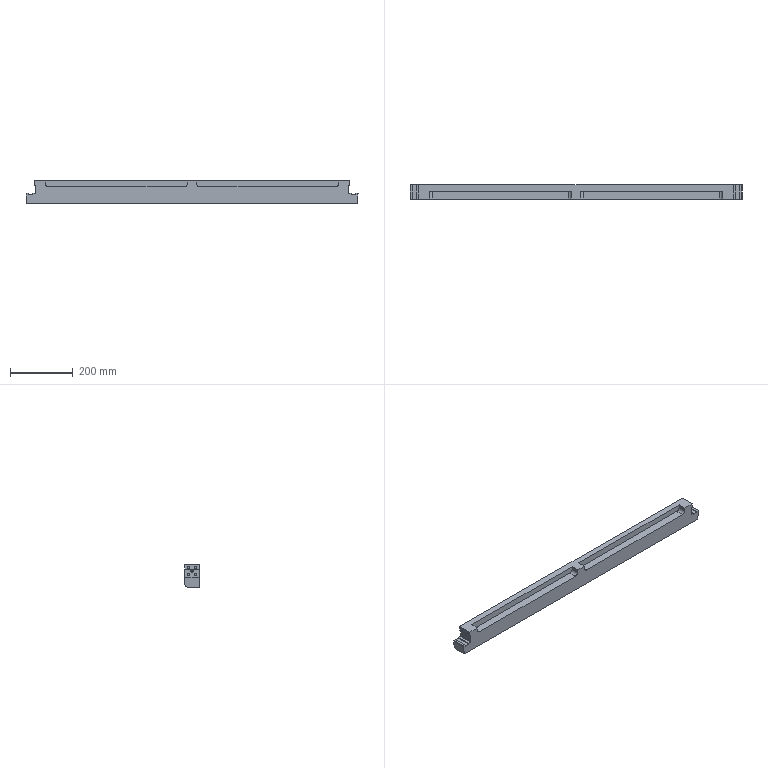NC program | NX | posted with a generic post | part box 1056 x 45 x 72.5 mm
Whole program:
N10 G17 G21 G94 G90
(ZLEVEL_PROFILE_COPY_1 , TOOL : D12)
N12 T20 M6
N14 G54
N16 G17 G0 G90 X532.563 Y44.63 B0. C0. S7500 M3
N18 G43 Z30. H20
N20 Z-1.
N22 G94 G1 X531.004 Y43.508 F3000.
N24 G3 X530.511 Y42.414 R1.2
N26 G1 X531.257 Y34.984
N28 X534.07 Y6.857
N30 X534.1 Y6.25
N32 Y4.25
N34 X534.096 Y3.509
N36 X534.097 Y-1.566
N38 G3 X534.697 Y-2.605 R1.2
N40 G1 X536.399 Y-3.588
N42 G0 Z-2.
N44 G1 X534.697 Y-2.605
N46 G2 X534.097 Y-1.566 R1.2
N48 G1 X534.096 Y3.509
N50 X534.1 Y4.25
N52 Y6.25
N54 X534.07 Y6.857
N56 X531.257 Y34.984
N58 X530.511 Y42.414
N60 G2 X531.004 Y43.508 R1.2
N62 G1 X532.563 Y44.63
N64 G0 Z-3.
N66 G1 X531.004 Y43.508
N68 G3 X530.511 Y42.414 R1.2
N70 G1 X531.257 Y34.984
N72 X534.07 Y6.857
N74 X534.1 Y6.25
N76 Y4.25
N78 X534.096 Y3.509
N80 X534.097 Y-1.566
N82 G3 X534.697 Y-2.605 R1.2
N84 G1 X536.399 Y-3.588
N86 G0 Z-4.
N88 G1 X534.697 Y-2.605
N90 G2 X534.097 Y-1.566 R1.2
N92 G1 X534.096 Y3.509
N94 X534.1 Y4.25
N96 Y6.25
N98 X534.07 Y6.857
N100 X531.257 Y34.984
N102 X530.511 Y42.414
N104 G2 X531.004 Y43.508 R1.2
N106 G1 X532.563 Y44.63
N108 G0 Z-5.
N110 G1 X531.004 Y43.508
N112 G3 X530.511 Y42.414 R1.2
N114 G1 X531.257 Y34.984
N116 X534.07 Y6.857
N118 X534.1 Y6.25
N120 Y4.25
N122 X534.096 Y3.509
N124 X534.097 Y-1.566
N126 G3 X534.697 Y-2.605 R1.2
N128 G1 X536.399 Y-3.588
N130 G0 Z-6.
N132 G1 X534.697 Y-2.605
N134 G2 X534.097 Y-1.566 R1.2
N136 G1 X534.096 Y3.509
N138 X534.1 Y4.25
N140 Y6.25
N142 X534.07 Y6.857
N144 X531.257 Y34.984
N146 X530.511 Y42.414
N148 G2 X531.004 Y43.508 R1.2
N150 G1 X532.563 Y44.63
N152 G0 Z-7.
N154 G1 X531.004 Y43.508
N156 G3 X530.511 Y42.414 R1.2
N158 G1 X531.257 Y34.984
N160 X534.07 Y6.857
N162 X534.1 Y6.25
N164 Y4.25
N166 X534.097 Y3.509
N168 Y-1.566
N170 G3 X534.697 Y-2.605 R1.2
N172 G1 X536.399 Y-3.588
N174 G0 Z-8.
N176 G1 X534.697 Y-2.605
N178 G2 X534.097 Y-1.566 R1.2
N180 G1 Y3.509
N182 X534.1 Y4.25
N184 Y6.25
N186 X534.07 Y6.857
N188 X531.257 Y34.984
N190 X530.511 Y42.414
N192 G2 X531.004 Y43.508 R1.2
N194 G1 X532.564 Y44.63
N196 G0 X532.571 Y44.635 Z-9.
N198 G1 X531.004 Y43.508
N200 G3 X530.511 Y42.414 R1.2
N202 G1 X531.257 Y34.984
N204 X534.07 Y6.857
N206 X534.1 Y6.25
N208 Y4.25
N210 X534.097 Y3.509
N212 Y-1.566
N214 G3 X534.697 Y-2.605 R1.2
N216 G1 X536.399 Y-3.588
N218 G0 X536.4 Z-10.
N220 G1 X534.697 Y-2.605
N222 G2 X534.097 Y-1.566 R1.2
N224 G1 Y3.509
N226 X534.1 Y4.25
N228 Y6.25
N230 X534.07 Y6.857
N232 X531.257 Y34.984
N234 X530.511 Y42.414
N236 G2 X531.005 Y43.508 R1.2
N238 G1 X532.571 Y44.635
N240 G0 Z-11.
N242 G1 X531.005 Y43.508
N244 G3 X530.511 Y42.414 R1.2
N246 G1 X531.257 Y34.984
N248 X534.07 Y6.857
N250 X534.1 Y6.25
N252 Y4.25
N254 X534.097 Y3.509
N256 Y-1.566
N258 G3 X534.697 Y-2.605 R1.2
N260 G1 X536.4 Y-3.588
N262 G0 Z-12.
N264 G1 X534.697 Y-2.605
N266 G2 X534.097 Y-1.566 R1.2
N268 G1 Y3.509
N270 X534.1 Y4.25
N272 Y6.25
N274 X534.07 Y6.857
N276 X531.257 Y34.984
N278 X530.511 Y42.414
N280 G2 X531.005 Y43.508 R1.2
N282 G1 X532.571 Y44.635
N284 G0 Z-13.
N286 G1 X531.005 Y43.508
N288 G3 X530.512 Y42.414 R1.2
N290 G1 X531.257 Y34.984
N292 X534.07 Y6.857
N294 X534.1 Y6.25
N296 Y4.25
N298 X534.097 Y3.509
N300 Y-1.566
N302 G3 X534.697 Y-2.605 R1.2
N304 G1 X536.4 Y-3.587
N306 G0 Z-14.
N308 G1 X534.698 Y-2.605
N310 G2 X534.097 Y-1.566 R1.2
N312 G1 Y3.509
N314 X534.1 Y4.25
N316 Y6.25
N318 X534.07 Y6.857
N320 X531.257 Y34.984
N322 X530.512 Y42.414
N324 G2 X531.005 Y43.508 R1.2
N326 G1 X532.571 Y44.635
N328 G0 Z-15.
N330 G1 X531.005 Y43.508
N332 G3 X530.512 Y42.414 R1.2
N334 G1 X531.257 Y34.984
N336 X534.07 Y6.857
N338 X534.1 Y6.25
N340 Y4.25
N342 X534.097 Y3.509
N344 Y-1.566
N346 G3 X534.698 Y-2.605 R1.2
N348 G1 X536.4 Y-3.587
N350 G0 Z-16.
N352 G1 X534.698 Y-2.605
N354 G2 X534.097 Y-1.566 R1.2
N356 G1 Y3.509
N358 X534.1 Y4.25
N360 Y6.25
N362 X534.07 Y6.857
N364 X531.257 Y34.984
N366 X530.512 Y42.414
N368 G2 X531.005 Y43.508 R1.2
N370 G1 X532.571 Y44.635
N372 G0 Y44.634 Z-17.
N374 G1 X531.005 Y43.508
N376 G3 X530.512 Y42.414 R1.2
N378 G1 X531.189 Y35.648
N380 X531.257 Y34.984
N382 X534.07 Y6.857
N384 X534.1 Y6.25
N386 Y4.25
N388 X534.097 Y3.509
N390 X534.098 Y-1.566
N392 G3 X534.698 Y-2.605 R1.2
N394 G1 X536.4 Y-3.587
N396 G0 Z-18.
N398 G1 X534.698 Y-2.605
N400 G2 X534.098 Y-1.566 R1.2
N402 G1 X534.097 Y3.509
N404 X534.1 Y4.25
N406 Y6.25
N408 X534.07 Y6.857
N410 X531.257 Y34.984
N412 X531.189 Y35.648
N414 X530.512 Y42.414
N416 G2 X531.006 Y43.508 R1.2
N418 G1 X532.571 Y44.634
N420 G0 Z-19.
N422 G1 X531.006 Y43.508
N424 G3 X530.512 Y42.414 R1.2
N426 G1 X531.189 Y35.648
N428 X531.257 Y34.984
N430 X534.07 Y6.857
N432 X534.1 Y6.25
N434 Y4.25
N436 X534.097 Y3.509
N438 X534.098 Y-1.566
N440 G3 X534.698 Y-2.605 R1.2
N442 G1 X536.4 Y-3.587
N444 G0 Z-20.
N446 G1 X534.698 Y-2.605
N448 G2 X534.098 Y-1.566 R1.2
N450 G1 X534.097 Y3.509
N452 X534.1 Y4.25
N454 Y6.25
N456 X534.07 Y6.857
N458 X531.257 Y34.984
N460 X531.189 Y35.648
N462 X530.512 Y42.414
N464 G2 X531.006 Y43.508 R1.2
N466 G1 X532.571 Y44.634
N468 G0 Z-21.
N470 G1 X531.006 Y43.508
N472 G3 X530.512 Y42.414 R1.2
N474 G1 X531.189 Y35.648
N476 X531.257 Y34.984
N478 X534.07 Y6.857
N480 X534.1 Y6.25
N482 Y4.25
N484 X534.097 Y3.509
N486 X534.098 Y-1.566
N488 G3 X534.698 Y-2.605 R1.2
N490 G1 X536.4 Y-3.587
N492 G0 Z-22.
N494 G1 X534.698 Y-2.605
N496 G2 X534.098 Y-1.566 R1.2
N498 G1 X534.097 Y3.509
N500 X534.1 Y4.25
N502 Y6.25
N504 X534.07 Y6.857
N506 X531.257 Y34.984
N508 X531.189 Y35.648
N510 X530.512 Y42.414
N512 G2 X531.006 Y43.508 R1.2
N514 G1 X532.571 Y44.634
N516 G0 X532.572 Z-23.
N518 G1 X531.006 Y43.508
N520 G3 X530.512 Y42.414 R1.2
N522 G1 X531.189 Y35.648
N524 X531.257 Y34.984
N526 X534.07 Y6.857
N528 X534.1 Y6.25
N530 Y4.25
N532 X534.097 Y3.509
N534 X534.098 Y-1.566
N536 G3 X534.698 Y-2.605 R1.2
N538 G1 X536.401 Y-3.587
N540 G0 Z-24.
N542 G1 X534.698 Y-2.605
N544 G2 X534.098 Y-1.566 R1.2
N546 G1 X534.097 Y3.509
N548 X534.1 Y4.25
N550 Y6.25
N552 X534.07 Y6.857
N554 X531.257 Y34.984
N556 X531.189 Y35.648
N558 X530.513 Y42.414
N560 G2 X531.006 Y43.508 R1.2
N562 G1 X532.572 Y44.634
N564 G0 Z-25.
N566 G1 X531.006 Y43.508
N568 G3 X530.513 Y42.414 R1.2
N570 G1 X531.189 Y35.648
N572 X531.257 Y34.984
N574 X534.07 Y6.857
N576 X534.1 Y6.25
N578 Y4.25
N580 X534.097 Y3.509
N582 X534.098 Y-1.566
N584 G3 X534.698 Y-2.605 R1.2
N586 G1 X536.401 Y-3.587
N588 G0 Z-26.
N590 G1 X534.698 Y-2.605
N592 G2 X534.098 Y-1.566 R1.2
N594 G1 X534.097 Y3.509
N596 X534.1 Y4.25
N598 Y6.25
N600 X534.07 Y6.857
N602 X531.251 Y35.029
N604 X530.513 Y42.414
N606 G2 X531.006 Y43.508 R1.2
N608 G1 X532.572 Y44.633
N610 G0 Y44.634 Z-27.
N612 G1 X531.006 Y43.508
N614 G3 X530.513 Y42.414 R1.2
N616 G1 X531.257 Y34.984
N618 X534.07 Y6.857
N620 X534.1 Y6.25
N622 Y4.25
N624 X534.097 Y3.509
N626 X534.098 Y-1.566
N628 G3 X534.698 Y-2.605 R1.2
N630 G1 X536.401 Y-3.587
N632 G0 Z-28.
N634 G1 X534.698 Y-2.605
N636 G2 X534.098 Y-1.566 R1.2
N638 G1 X534.097 Y3.509
N640 X534.1 Y4.25
N642 Y6.25
N644 X534.07 Y6.857
N646 X531.257 Y34.984
N648 X530.513 Y42.414
N650 G2 X531.006 Y43.508 R1.2
N652 G1 X532.572 Y44.634
N654 G0 Z-29.
N656 G1 X531.006 Y43.508
N658 G3 X530.513 Y42.414 R1.2
N660 G1 X531.257 Y34.984
N662 X534.07 Y6.857
N664 X534.1 Y6.25
N666 Y4.25
N668 X534.097 Y3.509
N670 X534.098 Y-1.566
N672 G3 X534.698 Y-2.605 R1.2
N674 G1 X536.401 Y-3.587
N676 G0 Z-30.
N678 G1 X534.699 Y-2.605
N680 G2 X534.098 Y-1.566 R1.2
N682 G1 X534.097 Y3.509
N684 X534.1 Y4.25
N686 Y6.25
N688 X534.07 Y6.857
N690 X531.257 Y34.984
N692 X530.513 Y42.414
N694 G2 X531.007 Y43.508 R1.2
N696 G1 X532.572 Y44.634
N698 G0 Z-31.
N700 G1 X531.007 Y43.508
N702 G3 X530.513 Y42.414 R1.2
N704 G1 X531.257 Y34.984
N706 X534.07 Y6.857
N708 X534.1 Y6.25
N710 Y4.25
N712 X534.097 Y3.509
N714 X534.098 Y-1.566
N716 G3 X534.699 Y-2.605 R1.2
N718 G1 X536.401 Y-3.587
N720 G0 Z-32.
N722 G1 X534.699 Y-2.605
N724 G2 X534.098 Y-1.566 R1.2
N726 G1 X534.097 Y3.509
N728 X534.1 Y4.25
N730 Y6.25
N732 X534.07 Y6.857
N734 X531.257 Y34.984
N736 X530.513 Y42.414
N738 G2 X531.007 Y43.508 R1.2
N740 G1 X532.572 Y44.634
N742 G0 Z-33.
N744 G1 X531.007 Y43.508
N746 G3 X530.513 Y42.415 R1.2
N748 G1 X531.257 Y34.984
N750 X534.07 Y6.857
N752 X534.1 Y6.25
N754 Y4.25
N756 X534.097 Y3.509
N758 X534.098 Y-1.566
N760 G3 X534.699 Y-2.605 R1.2
N762 G1 X536.401 Y-3.587
N764 G0 Z-34.
N766 G1 X534.699 Y-2.605
N768 G2 X534.098 Y-1.566 R1.2
N770 G1 X534.097 Y3.509
N772 X534.1 Y4.25
N774 Y6.25
N776 X534.07 Y6.857
N778 X531.257 Y34.984
N780 X530.513 Y42.415
N782 G2 X531.007 Y43.508 R1.2
N784 G1 X532.572 Y44.634
N786 G0 Y44.633 Z-35.
N788 G1 X531.007 Y43.508
N790 G3 X530.513 Y42.415 R1.2
N792 G1 X531.257 Y34.984
N794 X534.07 Y6.857
N796 X534.1 Y6.25
N798 Y4.25
N800 X534.097 Y3.509
N802 X534.098 Y-1.566
N804 G3 X534.699 Y-2.605 R1.2
N806 G1 X536.401 Y-3.587
N808 G0 Z-36.
N810 G1 X534.699 Y-2.605
N812 G2 X534.099 Y-1.566 R1.2
N814 G1 X534.097 Y3.509
N816 X534.1 Y4.25
N818 Y6.25
N820 X534.07 Y6.857
N822 X531.257 Y34.984
N824 X530.514 Y42.415
N826 G2 X531.007 Y43.508 R1.2
N828 G1 X532.572 Y44.633
N830 G0 Z-37.
N832 G1 X531.007 Y43.508
N834 G3 X530.514 Y42.415 R1.2
N836 G1 X531.257 Y34.984
N838 X534.07 Y6.857
N840 X534.1 Y6.25
N842 Y4.25
N844 X534.097 Y3.509
N846 X534.099 Y-1.566
N848 G3 X534.699 Y-2.605 R1.2
N850 G1 X536.402 Y-3.587
N852 G0 Z-38.
N854 G1 X534.699 Y-2.605
N856 G2 X534.099 Y-1.566 R1.2
N858 G1 X534.097 Y3.509
N860 X534.1 Y4.25
N862 Y6.25
N864 X534.07 Y6.857
N866 X531.257 Y34.984
N868 X530.514 Y42.415
N870 G2 X531.007 Y43.508 R1.2
N872 G1 X532.572 Y44.633
N874 G0 Z-39.
N876 G1 X531.007 Y43.508
N878 G3 X530.514 Y42.415 R1.2
N880 G1 X531.257 Y34.984
N882 X534.07 Y6.857
N884 X534.1 Y6.25
N886 Y4.25
N888 X534.097 Y3.509
N890 X534.099 Y-1.566
N892 G3 X534.699 Y-2.605 R1.2
N894 G1 X536.402 Y-3.587
N896 G0 Z-40.
N898 G1 X534.699 Y-2.605
N900 G2 X534.099 Y-1.566 R1.2
N902 G1 X534.097 Y3.509
N904 X534.1 Y4.25
N906 Y6.25
N908 X534.07 Y6.857
N910 X531.257 Y34.984
N912 X530.514 Y42.415
N914 G2 X531.008 Y43.508 R1.2
N916 G1 X532.572 Y44.633
N918 G0 Z-41.
N920 G1 X531.008 Y43.508
N922 G3 X530.514 Y42.415 R1.2
N924 G1 X531.257 Y34.984
N926 X534.07 Y6.857
N928 X534.1 Y6.25
N930 Y4.25
N932 X534.097 Y3.509
N934 X534.099 Y-1.566
N936 G3 X534.699 Y-2.605 R1.2
N938 G1 X536.402 Y-3.587
N940 G0 Z-42.
N942 G1 X534.699 Y-2.605
N944 G2 X534.099 Y-1.566 R1.2
N946 G1 X534.097 Y3.509
N948 X534.1 Y4.25
N950 Y6.25
N952 X534.07 Y6.857
N954 X531.257 Y34.984
N956 X530.514 Y42.415
N958 G2 X531.008 Y43.508 R1.2
N960 G1 X532.572 Y44.633
N962 G0 Z-43.
N964 G1 X531.008 Y43.508
N966 G3 X530.514 Y42.415 R1.2
N968 G1 X531.257 Y34.984
N970 X534.07 Y6.857
N972 X534.1 Y6.25
N974 Y4.25
N976 X534.097 Y3.509
N978 X534.099 Y-1.566
N980 G3 X534.699 Y-2.605 R1.2
N982 G1 X536.402 Y-3.587
N984 G0 Z-44.
N986 G1 X534.699 Y-2.605
N988 G2 X534.099 Y-1.566 R1.2
N990 G1 X534.097 Y3.509
N992 X534.1 Y4.25
N994 Y6.25
N996 X534.07 Y6.857
N998 X531.257 Y34.984
N1000 X530.514 Y42.415
N1002 G2 X531.008 Y43.508 R1.2
N1004 G1 X532.572 Y44.633
N1006 G0 Z-45.
N1008 G1 X531.008 Y43.508
N1010 G3 X530.514 Y42.415 R1.2
N1012 G1 X531.257 Y34.984
N1014 X534.07 Y6.857
N1016 X534.1 Y6.25
N1018 Y4.25
N1020 X534.097 Y3.509
N1022 X534.099 Y-1.566
N1024 G3 X534.699 Y-2.605 R1.2
N1026 G1 X536.402 Y-3.587
N1028 G0 Z30.
N1030 X-536.399 Y-3.588
N1032 Z-1.
N1034 G1 X-534.697 Y-2.605
N1036 G3 X-534.097 Y-1.566 R1.2
N1038 G1 X-534.096 Y3.35
N1040 X-534.1 Y4.204
N1042 Y6.25
N1044 G2 X-534.07 Y6.857 R6.1
N1046 G1 X-531.203 Y35.527
N1048 X-531.198 Y35.536
N1050 X-530.511 Y42.414
N1052 G3 X-531.004 Y43.508 R1.2
N1054 G1 X-532.576 Y44.638
N1056 G0 Z-2.
N1058 G1 X-531.004 Y43.508
N1060 G2 X-530.511 Y42.414 R1.2
N1062 G1 X-531.198 Y35.536
N1064 X-531.203 Y35.527
N1066 X-534.07 Y6.857
N1068 G3 X-534.1 Y6.25 R6.1
N1070 G1 Y4.204
N1072 X-534.096 Y3.35
N1074 X-534.097 Y-1.566
N1076 G2 X-534.697 Y-2.605 R1.2
N1078 G1 X-536.399 Y-3.588
N1080 G0 Z-3.
N1082 G1 X-534.697 Y-2.605
N1084 G3 X-534.097 Y-1.566 R1.2
N1086 G1 X-534.096 Y3.35
N1088 X-534.1 Y4.204
N1090 Y6.25
N1092 G2 X-534.07 Y6.857 R6.1
N1094 G1 X-531.203 Y35.527
N1096 X-531.198 Y35.536
N1098 X-530.511 Y42.414
N1100 G3 X-531.004 Y43.508 R1.2
N1102 G1 X-532.576 Y44.638
N1104 G0 Z-4.
N1106 G1 X-531.004 Y43.508
N1108 G2 X-530.511 Y42.414 R1.2
N1110 G1 X-531.198 Y35.536
N1112 X-531.203 Y35.527
N1114 X-534.07 Y6.857
N1116 G3 X-534.1 Y6.25 R6.1
N1118 G1 Y4.204
N1120 X-534.096 Y3.35
N1122 X-534.097 Y-1.566
N1124 G2 X-534.697 Y-2.605 R1.2
N1126 G1 X-536.399 Y-3.588
N1128 G0 Z-5.
N1130 G1 X-534.697 Y-2.605
N1132 G3 X-534.097 Y-1.566 R1.2
N1134 G1 X-534.096 Y3.35
N1136 X-534.1 Y4.204
N1138 Y6.25
N1140 G2 X-534.07 Y6.857 R6.1
N1142 G1 X-531.203 Y35.527
N1144 X-531.198 Y35.536
N1146 X-530.511 Y42.414
N1148 G3 X-531.005 Y43.508 R1.2
N1150 G1 X-532.576 Y44.638
N1152 G0 X-532.577 Z-6.
N1154 G1 X-531.005 Y43.508
N1156 G2 X-530.511 Y42.414 R1.2
N1158 G1 X-531.199 Y35.536
N1160 X-531.203 Y35.527
N1162 X-534.07 Y6.857
N1164 G3 X-534.1 Y6.25 R6.1
N1166 G1 Y4.204
N1168 X-534.096 Y3.35
N1170 X-534.097 Y-1.566
N1172 G2 X-534.697 Y-2.605 R1.2
N1174 G1 X-536.399 Y-3.588
N1176 G0 Z-7.
N1178 G1 X-534.697 Y-2.605
N1180 G3 X-534.097 Y-1.566 R1.2
N1182 G1 Y3.35
N1184 X-534.1 Y4.204
N1186 Y6.25
N1188 G2 X-534.07 Y6.857 R6.1
N1190 G1 X-531.203 Y35.527
N1192 X-531.199 Y35.536
N1194 X-530.511 Y42.414
N1196 G3 X-531.005 Y43.508 R1.2
N1198 G1 X-532.577 Y44.638
N1200 G0 Z-8.
N1202 G1 X-531.005 Y43.508
N1204 G2 X-530.511 Y42.414 R1.2
N1206 G1 X-531.199 Y35.536
N1208 X-531.203 Y35.527
N1210 X-534.07 Y6.857
N1212 G3 X-534.1 Y6.25 R6.1
N1214 G1 Y4.204
N1216 X-534.097 Y3.35
N1218 Y-1.566
N1220 G2 X-534.697 Y-2.605 R1.2
N1222 G1 X-536.399 Y-3.588
N1224 G0 Z-9.
N1226 G1 X-534.697 Y-2.605
N1228 G3 X-534.097 Y-1.566 R1.2
N1230 G1 Y3.35
N1232 X-534.1 Y4.204
N1234 Y6.25
N1236 G2 X-534.07 Y6.857 R6.1
N1238 G1 X-531.199 Y35.536
N1240 X-530.511 Y42.414
N1242 G3 X-531.005 Y43.508 R1.2
N1244 G1 X-532.577 Y44.638
N1246 G0 Z-10.
N1248 G1 X-531.005 Y43.508
N1250 G2 X-530.511 Y42.414 R1.2
N1252 G1 X-531.203 Y35.527
N1254 X-534.07 Y6.857
N1256 G3 X-534.1 Y6.25 R6.1
N1258 G1 Y4.204
N1260 X-534.097 Y3.35
N1262 Y-1.566
N1264 G2 X-534.697 Y-2.605 R1.2
N1266 G1 X-536.4 Y-3.588
N1268 G0 Z-11.
N1270 G1 X-534.697 Y-2.605
N1272 G3 X-534.097 Y-1.566 R1.2
N1274 G1 Y3.35
N1276 X-534.1 Y4.204
N1278 Y6.25
N1280 G2 X-534.07 Y6.857 R6.1
N1282 G1 X-531.199 Y35.536
N1284 X-530.511 Y42.414
N1286 G3 X-531.005 Y43.508 R1.2
N1288 G1 X-532.577 Y44.638
N1290 G0 Z-12.
N1292 G1 X-531.005 Y43.508
N1294 G2 X-530.511 Y42.414 R1.2
N1296 G1 X-531.203 Y35.527
N1298 X-534.07 Y6.857
N1300 G3 X-534.1 Y6.25 R6.1
N1302 G1 Y4.204
N1304 X-534.097 Y3.35
N1306 Y-1.566
N1308 G2 X-534.697 Y-2.605 R1.2
N1310 G1 X-536.4 Y-3.587
N1312 G0 Z-13.
N1314 G1 X-534.698 Y-2.605
N1316 G3 X-534.097 Y-1.566 R1.2
N1318 G1 Y3.35
N1320 X-534.1 Y4.204
N1322 Y6.25
N1324 G2 X-534.07 Y6.857 R6.1
N1326 G1 X-531.199 Y35.536
N1328 X-530.512 Y42.414
N1330 G3 X-531.005 Y43.508 R1.2
N1332 G1 X-532.577 Y44.638
N1334 G0 Z-14.
N1336 G1 X-531.005 Y43.508
N1338 G2 X-530.512 Y42.414 R1.2
N1340 G1 X-531.203 Y35.527
N1342 X-534.07 Y6.857
N1344 G3 X-534.1 Y6.25 R6.1
N1346 G1 Y4.204
N1348 X-534.097 Y3.35
N1350 Y-1.566
N1352 G2 X-534.698 Y-2.605 R1.2
N1354 G1 X-536.4 Y-3.587
N1356 G0 Z-15.
N1358 G1 X-534.698 Y-2.605
N1360 G3 X-534.097 Y-1.566 R1.2
N1362 G1 Y3.35
N1364 X-534.1 Y4.204
N1366 Y6.25
N1368 G2 X-534.07 Y6.857 R6.1
N1370 G1 X-531.199 Y35.536
N1372 X-530.512 Y42.414
N1374 G3 X-531.005 Y43.508 R1.2
N1376 G1 X-532.577 Y44.638
N1378 G0 X-532.578 Z-16.
N1380 G1 X-531.006 Y43.508
N1382 G2 X-530.512 Y42.414 R1.2
N1384 G1 X-531.203 Y35.527
N1386 X-534.07 Y6.857
N1388 G3 X-534.1 Y6.25 R6.1
N1390 G1 Y4.204
N1392 X-534.097 Y3.35
N1394 Y-1.566
N1396 G2 X-534.698 Y-2.605 R1.2
N1398 G1 X-536.4 Y-3.587
N1400 G0 Z-17.
N1402 G1 X-534.698 Y-2.605
N1404 G3 X-534.098 Y-1.566 R1.2
N1406 G1 X-534.097 Y3.35
N1408 X-534.1 Y4.204
N1410 Y6.25
N1412 G2 X-534.07 Y6.857 R6.1
N1414 G1 X-531.199 Y35.536
N1416 X-530.512 Y42.414
N1418 G3 X-531.006 Y43.508 R1.2
N1420 G1 X-532.578 Y44.638
N1422 G0 Z-18.
N1424 G1 X-531.006 Y43.508
N1426 G2 X-530.512 Y42.414 R1.2
N1428 G1 X-531.203 Y35.527
N1430 X-534.07 Y6.857
N1432 G3 X-534.1 Y6.25 R6.1
N1434 G1 Y4.204
N1436 X-534.097 Y3.35
N1438 X-534.098 Y-1.566
N1440 G2 X-534.698 Y-2.605 R1.2
N1442 G1 X-536.4 Y-3.587
N1444 G0 Z-19.
N1446 G1 X-534.698 Y-2.605
N1448 G3 X-534.098 Y-1.566 R1.2
N1450 G1 X-534.097 Y3.35
N1452 X-534.1 Y4.204
N1454 Y6.25
N1456 G2 X-534.07 Y6.857 R6.1
N1458 G1 X-531.2 Y35.536
N1460 X-530.512 Y42.414
N1462 G3 X-531.006 Y43.508 R1.2
N1464 G1 X-532.578 Y44.638
N1466 G0 Y44.639 Z-20.
N1468 G1 X-531.006 Y43.508
N1470 G2 X-530.512 Y42.414 R1.2
N1472 G1 X-531.203 Y35.514
N1474 X-531.323 Y34.326
N1476 X-534.07 Y6.857
N1478 G3 X-534.1 Y6.25 R6.1
N1480 G1 Y4.204
N1482 X-534.097 Y3.35
N1484 X-534.098 Y-1.566
N1486 G2 X-534.698 Y-2.605 R1.2
N1488 G1 X-536.4 Y-3.587
N1490 G0 Z-21.
N1492 G1 X-534.698 Y-2.605
N1494 G3 X-534.098 Y-1.566 R1.2
N1496 G1 X-534.097 Y3.35
N1498 X-534.1 Y4.204
N1500 Y6.25
N1502 G2 X-534.07 Y6.857 R6.1
N1504 G1 X-531.323 Y34.326
N1506 X-531.203 Y35.514
N1508 X-530.512 Y42.414
N1510 G3 X-531.006 Y43.508 R1.2
N1512 G1 X-532.578 Y44.639
N1514 G0 Z-22.
N1516 G1 X-531.006 Y43.508
N1518 G2 X-530.512 Y42.414 R1.2
N1520 G1 X-531.203 Y35.514
N1522 X-531.323 Y34.326
N1524 X-534.07 Y6.857
N1526 G3 X-534.1 Y6.25 R6.1
N1528 G1 Y4.204
N1530 X-534.097 Y3.35
N1532 X-534.098 Y-1.566
N1534 G2 X-534.698 Y-2.605 R1.2
N1536 G1 X-536.4 Y-3.587
N1538 G0 X-536.401 Z-23.
N1540 G1 X-534.698 Y-2.605
N1542 G3 X-534.098 Y-1.566 R1.2
N1544 G1 X-534.097 Y3.35
N1546 X-534.1 Y4.204
N1548 Y6.25
N1550 G2 X-534.07 Y6.857 R6.1
N1552 G1 X-531.323 Y34.326
N1554 X-531.203 Y35.514
N1556 X-530.512 Y42.414
N1558 G3 X-531.006 Y43.508 R1.2
N1560 G1 X-532.578 Y44.639
N1562 G0 Y44.638 Z-24.
N1564 G1 X-531.006 Y43.508
N1566 G2 X-530.513 Y42.414 R1.2
N1568 G1 X-531.274 Y34.802
N1570 X-531.323 Y34.326
N1572 X-534.07 Y6.857
N1574 G3 X-534.1 Y6.25 R6.1
N1576 G1 Y4.204
N1578 X-534.097 Y3.35
N1580 X-534.098 Y-1.566
N1582 G2 X-534.698 Y-2.605 R1.2
N1584 G1 X-536.401 Y-3.587
N1586 G0 Z-25.
N1588 G1 X-534.698 Y-2.605
N1590 G3 X-534.098 Y-1.566 R1.2
N1592 G1 X-534.097 Y3.35
N1594 X-534.1 Y4.204
N1596 Y6.25
N1598 G2 X-534.07 Y6.857 R6.1
N1600 G1 X-531.323 Y34.326
N1602 X-530.513 Y42.414
N1604 G3 X-531.006 Y43.508 R1.2
N1606 G1 X-532.578 Y44.639
N1608 G0 Z-26.
N1610 G1 X-531.006 Y43.508
N1612 G2 X-530.513 Y42.414 R1.2
N1614 G1 X-531.323 Y34.326
N1616 X-534.07 Y6.857
N1618 G3 X-534.1 Y6.25 R6.1
N1620 G1 Y4.204
N1622 X-534.097 Y3.35
N1624 X-534.098 Y-1.566
N1626 G2 X-534.698 Y-2.605 R1.2
N1628 G1 X-536.401 Y-3.587
N1630 G0 Z-27.
N1632 G1 X-534.698 Y-2.605
N1634 G3 X-534.098 Y-1.566 R1.2
N1636 G1 X-534.097 Y3.35
N1638 X-534.1 Y4.204
N1640 Y6.25
N1642 G2 X-534.07 Y6.857 R6.1
N1644 G1 X-531.323 Y34.326
N1646 X-530.513 Y42.414
N1648 G3 X-531.006 Y43.508 R1.2
N1650 G1 X-532.578 Y44.639
N1652 G0 X-532.579 Z-28.
N1654 G1 X-531.006 Y43.508
N1656 G2 X-530.513 Y42.414 R1.2
N1658 G1 X-531.323 Y34.326
N1660 X-534.07 Y6.857
N1662 G3 X-534.1 Y6.25 R6.1
N1664 G1 Y4.204
N1666 X-534.097 Y3.35
N1668 X-534.098 Y-1.566
N1670 G2 X-534.698 Y-2.605 R1.2
N1672 G1 X-536.401 Y-3.587
N1674 G0 Z-29.
N1676 G1 X-534.698 Y-2.605
N1678 G3 X-534.098 Y-1.566 R1.2
N1680 G1 X-534.097 Y3.35
N1682 X-534.1 Y4.204
N1684 Y6.25
N1686 G2 X-534.07 Y6.857 R6.1
N1688 G1 X-531.323 Y34.326
N1690 X-530.513 Y42.414
N1692 G3 X-531.006 Y43.508 R1.2
N1694 G1 X-532.579 Y44.639
N1696 G0 Z-30.
N1698 G1 X-531.007 Y43.508
N1700 G2 X-530.513 Y42.414 R1.2
N1702 G1 X-531.323 Y34.326
N1704 X-534.07 Y6.857
N1706 G3 X-534.1 Y6.25 R6.1
N1708 G1 Y4.204
N1710 X-534.097 Y3.35
N1712 X-534.098 Y-1.566
N1714 G2 X-534.699 Y-2.605 R1.2
N1716 G1 X-536.401 Y-3.587
N1718 G0 Z-31.
N1720 G1 X-534.699 Y-2.605
N1722 G3 X-534.098 Y-1.566 R1.2
N1724 G1 X-534.097 Y3.35
N1726 X-534.1 Y4.204
N1728 Y6.25
N1730 G2 X-534.07 Y6.857 R6.1
N1732 G1 X-531.323 Y34.326
N1734 X-530.513 Y42.414
N1736 G3 X-531.007 Y43.508 R1.2
N1738 G1 X-532.579 Y44.639
N1740 G0 Z-32.
N1742 G1 X-531.007 Y43.508
N1744 G2 X-530.513 Y42.414 R1.2
N1746 G1 X-531.323 Y34.326
N1748 X-534.07 Y6.857
N1750 G3 X-534.1 Y6.25 R6.1
N1752 G1 Y4.204
N1754 X-534.097 Y3.35
N1756 X-534.098 Y-1.566
N1758 G2 X-534.699 Y-2.605 R1.2
N1760 G1 X-536.401 Y-3.587
N1762 G0 Z-33.
N1764 G1 X-534.699 Y-2.605
N1766 G3 X-534.098 Y-1.566 R1.2
N1768 G1 X-534.097 Y3.35
N1770 X-534.1 Y4.204
N1772 Y6.25
N1774 G2 X-534.07 Y6.857 R6.1
N1776 G1 X-531.323 Y34.326
N1778 X-530.513 Y42.415
N1780 G3 X-531.007 Y43.508 R1.2
N1782 G1 X-532.579 Y44.639
N1784 G0 Z-34.
N1786 G1 X-531.007 Y43.508
N1788 G2 X-530.513 Y42.415 R1.2
N1790 G1 X-531.323 Y34.326
N1792 X-534.07 Y6.857
N1794 G3 X-534.1 Y6.25 R6.1
N1796 G1 Y4.204
N1798 X-534.097 Y3.35
N1800 X-534.098 Y-1.566
N1802 G2 X-534.699 Y-2.605 R1.2
N1804 G1 X-536.401 Y-3.587
N1806 G0 Z-35.
N1808 G1 X-534.699 Y-2.605
N1810 G3 X-534.098 Y-1.566 R1.2
N1812 G1 X-534.097 Y3.35
N1814 X-534.1 Y4.204
N1816 Y6.25
N1818 G2 X-534.07 Y6.857 R6.1
N1820 G1 X-531.323 Y34.326
N1822 X-530.513 Y42.415
N1824 G3 X-531.007 Y43.508 R1.2
N1826 G1 X-532.579 Y44.639
N1828 G0 Z-36.
N1830 G1 X-531.007 Y43.508
N1832 G2 X-530.514 Y42.415 R1.2
N1834 G1 X-531.323 Y34.326
N1836 X-534.07 Y6.857
N1838 G3 X-534.1 Y6.25 R6.1
N1840 G1 Y4.204
N1842 X-534.097 Y3.35
N1844 X-534.099 Y-1.566
N1846 G2 X-534.699 Y-2.605 R1.2
N1848 G1 X-536.402 Y-3.587
N1850 G0 Z-37.
N1852 G1 X-534.699 Y-2.605
N1854 G3 X-534.099 Y-1.566 R1.2
N1856 G1 X-534.097 Y3.35
N1858 X-534.1 Y4.204
N1860 Y6.25
N1862 G2 X-534.07 Y6.857 R6.1
N1864 G1 X-531.323 Y34.326
N1866 X-530.514 Y42.415
N1868 G3 X-531.007 Y43.508 R1.2
N1870 G1 X-532.58 Y44.639
N1872 G0 Z-38.
N1874 G1 X-531.007 Y43.508
N1876 G2 X-530.514 Y42.415 R1.2
N1878 G1 X-531.323 Y34.326
N1880 X-534.07 Y6.857
N1882 G3 X-534.1 Y6.25 R6.1
N1884 G1 Y4.204
N1886 X-534.097 Y3.35
N1888 X-534.099 Y-1.566
N1890 G2 X-534.699 Y-2.605 R1.2
N1892 G1 X-536.402 Y-3.587
N1894 G0 Z-39.
N1896 G1 X-534.699 Y-2.605
N1898 G3 X-534.099 Y-1.566 R1.2
N1900 G1 X-534.097 Y3.35
N1902 X-534.1 Y4.204
N1904 Y6.25
N1906 G2 X-534.07 Y6.857 R6.1
N1908 G1 X-531.323 Y34.326
N1910 X-530.514 Y42.415
N1912 G3 X-531.007 Y43.508 R1.2
N1914 G1 X-532.58 Y44.639
N1916 G0 Z-40.
N1918 G1 X-531.008 Y43.508
N1920 G2 X-530.514 Y42.415 R1.2
N1922 G1 X-531.202 Y35.533
N1924 X-534.07 Y6.857
N1926 G3 X-534.1 Y6.25 R6.1
N1928 G1 Y4.204
N1930 G3 X-534.042 Y3.411 R6.1
N1932 G1 X-534.097 Y3.35
N1934 X-534.099 Y-1.566
N1936 G2 X-534.699 Y-2.605 R1.2
N1938 G1 X-536.402 Y-3.587
N1940 G0 Z-41.
N1942 G1 X-534.699 Y-2.605
N1944 G3 X-534.099 Y-1.566 R1.2
N1946 G1 X-534.097 Y3.35
N1948 X-534.042 Y3.411
N1950 G2 X-534.1 Y4.25 R6.1
N1952 G1 Y6.25
N1954 G2 X-534.07 Y6.857 R6.1
N1956 G1 X-531.202 Y35.533
N1958 X-530.514 Y42.415
N1960 G3 X-531.008 Y43.508 R1.2
N1962 G1 X-532.58 Y44.639
N1964 G0 Z-42.
N1966 G1 X-531.008 Y43.508
N1968 G2 X-530.514 Y42.415 R1.2
N1970 G1 X-531.202 Y35.533
N1972 X-534.07 Y6.857
N1974 G3 X-534.1 Y6.25 R6.1
N1976 G1 Y4.204
N1978 G3 X-534.042 Y3.411 R6.1
N1980 G1 X-534.097 Y3.35
N1982 X-534.099 Y-1.566
N1984 G2 X-534.699 Y-2.605 R1.2
N1986 G1 X-536.402 Y-3.587
N1988 G0 Z-43.
N1990 G1 X-534.699 Y-2.605
N1992 G3 X-534.099 Y-1.566 R1.2
N1994 G1 X-534.097 Y3.35
N1996 X-534.042 Y3.411
N1998 G2 X-534.1 Y4.25 R6.1
N2000 G1 Y6.25
N2002 G2 X-534.07 Y6.857 R6.1
N2004 G1 X-531.202 Y35.533
N2006 X-530.514 Y42.415
N2008 G3 X-531.008 Y43.508 R1.2
N2010 G1 X-532.58 Y44.639
N2012 G0 Z-44.
N2014 G1 X-531.008 Y43.508
N2016 G2 X-530.514 Y42.415 R1.2
N2018 G1 X-531.202 Y35.533
N2020 X-534.07 Y6.857
N2022 G3 X-534.1 Y6.25 R6.1
N2024 G1 Y4.204
N2026 G3 X-534.042 Y3.411 R6.1
N2028 G1 X-534.097 Y3.35
N2030 X-534.099 Y-1.566
N2032 G2 X-534.699 Y-2.605 R1.2
N2034 G1 X-536.402 Y-3.587
N2036 G0 Z-45.
N2038 G1 X-534.699 Y-2.605
N2040 G3 X-534.099 Y-1.566 R1.2
N2042 G1 X-534.097 Y3.35
N2044 X-534.042 Y3.411
N2046 G2 X-534.1 Y4.25 R6.1
N2048 G1 Y6.25
N2050 G2 X-534.07 Y6.857 R6.1
N2052 G1 X-531.202 Y35.533
N2054 X-530.514 Y42.415
N2056 G3 X-531.008 Y43.508 R1.2
N2058 G1 X-532.58 Y44.639
N2060 G0 Z30.
N2062 M5
(111 , TOOL : D12JING)
N2064 T21 M6
N2066 G54
N2068 G17 G0 G90 X524.294 Y47.768 B0. C0. S6500 M3
N2070 G43 Z30. H21
N2072 Z-14.
N2074 G94 G1 Z-15. F1000.
N2076 G41 X524.227 Y47.693 D21
N2078 X523.519 Y46.566
N2080 G3 X523.73 Y45.038 R1.2
N2082 G1 X528.844 Y40.411
N2084 X529.076 Y40.201
N2086 G2 X531.02 Y36.35 R6.
N2088 G1 X533.97 Y6.847
N2090 X534. Y6.25
N2092 Y4.789
N2094 X534.002 Y4.765
N2096 X533.978 Y4.76
N2098 G2 X532.243 Y0.007 R6.
N2100 G1 X531.743 Y-0.493
N2102 X531.379 Y-0.854
N2104 X527.195 Y-5.038
N2106 G3 X527.06 Y-6.575 R1.2
N2108 G1 X527.828 Y-7.671
N2110 G40
N2112 X527.899 Y-7.742
N2114 Z-14.
N2116 G0 Z30.
N2118 X524.295 Y47.768
N2120 Z-29.
N2122 G1 Z-30.
N2124 G41 X524.227 Y47.694
N2126 X523.519 Y46.567
N2128 G3 X523.73 Y45.038 R1.2
N2130 G1 X528.844 Y40.411
N2132 X529.076 Y40.201
N2134 G2 X531.02 Y36.35 R6.
N2136 G1 X533.97 Y6.847
N2138 X534. Y6.25
N2140 Y4.789
N2142 X534.002 Y4.765
N2144 X533.978 Y4.76
N2146 G2 X532.243 Y0.007 R6.
N2148 G1 X531.743 Y-0.493
N2150 X531.379 Y-0.855
N2152 X527.196 Y-5.038
N2154 G3 X527.061 Y-6.575 R1.2
N2156 G1 X527.828 Y-7.671
N2158 G40
N2160 X527.899 Y-7.742
N2162 Z-29.
N2164 G0 Z30.
N2166 X524.295 Y47.768
N2168 Z-44.
N2170 G1 Z-45.
N2172 G41 X524.228 Y47.694
N2174 X523.52 Y46.567
N2176 G3 X523.73 Y45.039 R1.2
N2178 G1 X528.844 Y40.411
N2180 X529.076 Y40.201
N2182 G2 X531.02 Y36.35 R6.
N2184 G1 X533.97 Y6.847
N2186 X534. Y6.25
N2188 Y4.868
N2190 X533.999 Y4.762
N2192 X533.98 Y4.745
N2194 G2 X532.243 Y0.007 R6.
N2196 G1 X531.743 Y-0.493
N2198 X527.196 Y-5.039
N2200 G3 X527.061 Y-6.576 R1.2
N2202 G1 X527.829 Y-7.672
N2204 G40
N2206 X527.9 Y-7.743
N2208 Z-44.
N2210 G0 Z30.
N2212 X-527.898 Y-7.741
N2214 Z-14.
N2216 G1 Z-15.
N2218 G41 X-527.828 Y-7.671
N2220 X-527.06 Y-6.574
N2222 G3 X-527.195 Y-5.038 R1.2
N2224 G1 X-531.474 Y-0.758
N2226 X-531.743 Y-0.493
N2228 X-531.775 Y-0.46
N2230 X-531.781 Y-0.449
N2232 X-531.868 Y-0.366
N2234 X-531.857 Y-0.346
N2236 G2 X-534. Y4.25 R6.
N2238 G1 Y6.25
N2240 G2 X-533.97 Y6.847 R6.
N2242 G1 X-531.02 Y36.35
N2244 G2 X-529.076 Y40.201 R6.
N2246 G1 X-528.81 Y40.442
N2248 X-523.73 Y45.038
N2250 G3 X-523.518 Y46.566 R1.2
N2252 G1 X-524.227 Y47.693
N2254 G40
N2256 X-524.294 Y47.767
N2258 Z-14.
N2260 G0 Z30.
N2262 X-527.898 Y-7.742
N2264 Z-29.
N2266 G1 Z-30.
N2268 G41 X-527.827 Y-7.671
N2270 X-527.06 Y-6.575
N2272 G3 X-527.195 Y-5.038 R1.2
N2274 G1 X-531.743 Y-0.493
N2276 X-531.775 Y-0.46
N2278 X-531.781 Y-0.449
N2280 X-531.868 Y-0.367
N2282 X-531.857 Y-0.346
N2284 G2 X-534. Y4.25 R6.
N2286 G1 Y6.25
N2288 G2 X-533.97 Y6.847 R6.
N2290 G1 X-531.02 Y36.35
N2292 G2 X-529.076 Y40.201 R6.
N2294 G1 X-528.81 Y40.442
N2296 X-523.73 Y45.038
N2298 G3 X-523.519 Y46.566 R1.2
N2300 G1 X-524.227 Y47.694
N2302 G40
N2304 X-524.294 Y47.768
N2306 Z-29.
N2308 G0 Z30.
N2310 X-527.898 Y-7.742
N2312 Z-44.
N2314 G1 Z-45.
N2316 G41 X-527.828 Y-7.671
N2318 X-527.06 Y-6.575
N2320 G3 X-527.195 Y-5.038 R1.2
N2322 G1 X-531.743 Y-0.493
N2324 X-531.775 Y-0.46
N2326 X-531.782 Y-0.449
N2328 X-531.868 Y-0.367
N2330 X-531.857 Y-0.346
N2332 G2 X-534. Y4.25 R6.
N2334 G1 Y6.25
N2336 G2 X-533.97 Y6.847 R6.
N2338 G1 X-531.02 Y36.35
N2340 G2 X-529.076 Y40.201 R6.
N2342 G1 X-528.81 Y40.442
N2344 X-528.448 Y40.768
N2346 X-523.73 Y45.038
N2348 G3 X-523.519 Y46.566 R1.2
N2350 G1 X-524.228 Y47.694
N2352 G40
N2354 X-524.295 Y47.768
N2356 Z-44.
N2358 G0 Z30.
N2360 M5
(FLOOR_WALL_1 , TOOL : D10)
N2362 T10 M6
N2364 G54
N2366 G17 G0 G90 X-38.519 Y-44.25 B0. C0. S7500 M3
N2368 G43 Z30. H10
N2370 Z-21.85
N2372 G94 G1 Z-24.85 F1000.
N2374 X-39.053 Y-41.25
N2376 G2 X-39.157 Y-40.6 R19.2 F3000.
N2378 G1 X-441.843
N2380 G2 X-441.948 Y-41.25 R19.2
N2382 G1 X-442.761
N2384 G3 X-442.55 Y-39.8 R18.4
N2386 G1 X-38.45
N2388 G3 X-38.24 Y-41.25 R18.4
N2390 G1 X-37.426
N2392 G2 X-37.715 Y-39. R17.6
N2394 G1 X-443.285
N2396 G2 X-443.575 Y-41.25 R17.6
N2398 G1 X-444.391
N2400 G3 X-444.053 Y-38.2 R16.8
N2402 G1 X-36.947
N2404 G3 X-36.61 Y-41.25 R16.8
N2406 G1 X-35.792
N2408 G2 X-36.15 Y-37.877 R16.
N2410 G1 Y-37.4
N2412 X-444.85
N2414 Y-37.883
N2416 G2 X-445.208 Y-41.25 R16.
N2418 G1 X-446.028
N2420 G3 X-445.65 Y-37.883 R15.2
N2422 G1 Y-36.6
N2424 X-35.35
N2426 Y-37.877
N2428 G3 X-34.973 Y-41.25 R15.2
N2430 G1 X-34.152
N2432 G2 X-34.55 Y-37.877 R14.4
N2434 G1 Y-35.8
N2436 X-446.45
N2438 Y-37.883
N2440 G2 X-446.849 Y-41.25 R14.4
N2442 G1 X-447.673
N2444 G3 X-447.25 Y-37.883 R13.6
N2446 G1 Y-35.
N2448 X-33.75
N2450 Y-37.877
N2452 G3 X-33.328 Y-41.25 R13.6
N2454 G1 X-32.5
N2456 G2 X-32.95 Y-37.877 R12.8
N2458 G1 Y-34.2
N2460 X-448.05
N2462 Y-37.883
N2464 G2 X-448.501 Y-41.25 R12.8
N2466 G1 X-449.332
N2468 G3 X-448.85 Y-37.883 R12.
N2470 G1 Y-33.4
N2472 X-32.15
N2474 Y-37.877
N2476 G3 X-31.669 Y-41.25 R12.
N2478 G1 X-30.833
N2480 G2 X-31.35 Y-37.877 R11.2
N2482 G1 Y-32.6
N2484 X-449.65
N2486 Y-37.883
N2488 G2 X-450.168 Y-41.25 R11.2
N2490 G1 X-451.01
N2492 G3 X-450.45 Y-37.883 R10.4
N2494 G1 Y-31.8
N2496 X-30.55
N2498 Y-37.877
N2500 G3 X-29.991 Y-41.25 R10.4
N2502 G1 X-29.142
N2504 G2 X-29.75 Y-37.877 R9.6
N2506 G1 Y-31.
N2508 X-451.25
N2510 Y-37.883
N2512 G2 X-451.86 Y-41.25 R9.6
N2514 G1 X-452.72
N2516 G3 X-452.05 Y-37.883 R8.8
N2518 G1 Y-30.2
N2520 X-28.95
N2522 Y-37.877
N2524 G3 X-28.282 Y-41.25 R8.8
N2526 G1 X-27.409
N2528 G2 X-28.15 Y-37.878 R8.
N2530 G1 Y-29.4
N2532 X-452.85
N2534 Y-37.883
N2536 G2 X-453.593 Y-41.25 R8.
N2538 G1 X-454.486
N2540 G3 X-453.65 Y-37.883 R7.2
N2542 G1 Y-28.6
N2544 X-27.35
N2546 Y-37.878
N2548 G3 X-26.516 Y-41.25 R7.2
N2550 G1 X-25.595
N2552 G2 X-26.55 Y-37.878 R6.4
N2554 G1 Y-27.8
N2556 X-454.45
N2558 Y-37.883
N2560 G2 X-455.407 Y-41.25 R6.4
N2562 G1 X-456.375
N2564 G3 X-455.25 Y-37.883 R5.6
N2566 G1 Y-27.
N2568 X-25.75
N2570 Y-37.879
N2572 G3 X-24.627 Y-41.25 R5.6
N2574 G1 X-23.571
N2576 X-23.648 Y-41.174
N2578 G2 X-24.95 Y-37.879 R4.8
N2580 G1 Y-26.25
N2582 X-24.947 Y-26.197
N2584 X-25. Y-26.2
N2586 X-456.
N2588 X-456.053 Y-26.197
N2590 X-456.05 Y-26.25
N2592 Y-37.883
N2594 G2 X-457.429 Y-41.25 R4.8
N2596 G1 X-458.56
N2598 X-458.022 Y-40.712
N2600 G3 X-456.85 Y-37.883 R4.
N2602 G1 Y-26.25
N2604 G2 X-456. Y-25.4 R0.85
N2606 G1 X-25.
N2608 G2 X-24.15 Y-26.25 R0.85
N2610 G1 Y-37.88
N2612 G3 X-23.072 Y-40.618 R4.
N2614 G1 X-22.44 Y-41.25
N2616 X-21.309
N2618 X-22.496 Y-40.063
N2620 G2 X-23.35 Y-37.88 R3.2
N2622 G1 Y-26.25
N2624 G3 X-25. Y-24.6 R1.65
N2626 G1 X-456.
N2628 G3 X-457.65 Y-26.25 R1.65
N2630 G1 Y-37.883
N2632 G2 X-458.587 Y-40.146 R3.2
N2634 G1 X-459.691 Y-41.25
N2636 X-460.823
N2638 X-459.153 Y-39.58
N2640 G3 X-458.45 Y-37.883 R2.4
N2642 G1 Y-26.25
N2644 G2 X-456. Y-23.8 R2.45
N2646 G1 X-25.
N2648 G2 X-22.55 Y-26.25 R2.45
N2650 G1 Y-37.881
N2652 G3 X-21.918 Y-39.509 R2.4
N2654 G1 X-20.177 Y-41.25
N2656 X-19.046
N2658 X-21.338 Y-38.958
N2660 G2 X-21.75 Y-37.882 R1.6
N2662 G1 Y-26.25
N2664 G3 X-25. Y-23. R3.25
N2666 G1 X-456.
N2668 G3 X-459.25 Y-26.25 R3.25
N2670 G1 Y-37.883
N2672 G2 X-459.719 Y-39.015 R1.6
N2674 G1 X-461.954 Y-41.25
N2676 X-463.085
N2678 X-460.284 Y-38.449
N2680 G3 X-460.05 Y-37.883 R0.8
N2682 G1 Y-26.25
N2684 G2 X-456. Y-22.2 R4.05
N2686 G1 X-25.
N2688 G2 X-20.95 Y-26.25 R4.05
N2690 G1 Y-37.883
N2692 G3 X-20.753 Y-38.412 R0.8
N2694 G1 X-17.915 Y-41.25
N2696 X-16.813
N2698 Y-41.22
N2700 X-20.15 Y-37.883
N2702 Y-26.25
N2704 G3 X-25. Y-21.4 R4.85
N2706 G1 X-456.
N2708 G3 X-460.85 Y-26.25 R4.85
N2710 G1 Y-37.883
N2712 X-464.217 Y-41.25
N2714 X-467.367 Y-44.4
N2716 Z-21.85
N2718 G0 Z30.
N2720 X442.481 Y-44.25
N2722 Z-21.85
N2724 G1 Z-24.85 F1000.
N2726 X441.947 Y-41.25
N2728 G2 X441.843 Y-40.6 R19.2 F3000.
N2730 G1 X39.157
N2732 G2 X39.053 Y-41.25 R19.2
N2734 G1 X38.239
N2736 G3 X38.45 Y-39.8 R18.4
N2738 G1 X442.55
N2740 G3 X442.76 Y-41.25 R18.4
N2742 G1 X443.574
N2744 G2 X443.285 Y-39. R17.6
N2746 G1 X37.715
N2748 G2 X37.425 Y-41.25 R17.6
N2750 G1 X36.609
N2752 G3 X36.947 Y-38.2 R16.8
N2754 G1 X444.053
N2756 G3 X444.39 Y-41.25 R16.8
N2758 G1 X445.208
N2760 G2 X444.85 Y-37.876 R16.
N2762 G1 Y-37.4
N2764 X36.15
N2766 Y-37.883
N2768 G2 X35.792 Y-41.25 R16.
N2770 G1 X34.972
N2772 G3 X35.35 Y-37.883 R15.2
N2774 G1 Y-36.6
N2776 X445.65
N2778 Y-37.876
N2780 G3 X446.027 Y-41.25 R15.2
N2782 G1 X446.848
N2784 G2 X446.45 Y-37.876 R14.4
N2786 G1 Y-35.8
N2788 X34.55
N2790 Y-37.883
N2792 G2 X34.151 Y-41.25 R14.4
N2794 G1 X33.327
N2796 G3 X33.75 Y-37.883 R13.6
N2798 G1 Y-35.
N2800 X447.25
N2802 Y-37.876
N2804 G3 X447.672 Y-41.25 R13.6
N2806 G1 X448.5
N2808 G2 X448.05 Y-37.876 R12.8
N2810 G1 Y-34.2
N2812 X32.95
N2814 Y-37.883
N2816 G2 X32.499 Y-41.25 R12.8
N2818 G1 X31.668
N2820 G3 X32.15 Y-37.883 R12.
N2822 G1 Y-33.4
N2824 X448.85
N2826 Y-37.876
N2828 G3 X449.331 Y-41.25 R12.
N2830 G1 X450.167
N2832 G2 X449.65 Y-37.876 R11.2
N2834 G1 Y-32.6
N2836 X31.35
N2838 Y-37.883
N2840 G2 X30.832 Y-41.25 R11.2
N2842 G1 X29.99
N2844 G3 X30.55 Y-37.883 R10.4
N2846 G1 Y-31.8
N2848 X450.45
N2850 Y-37.876
N2852 G3 X451.009 Y-41.25 R10.4
N2854 G1 X451.859
N2856 G2 X451.25 Y-37.876 R9.6
N2858 G1 Y-31.
N2860 X29.75
N2862 Y-37.883
N2864 G2 X29.14 Y-41.25 R9.6
N2866 G1 X28.28
N2868 G3 X28.95 Y-37.883 R8.8
N2870 G1 Y-30.2
N2872 X452.05
N2874 Y-37.877
N2876 G3 X452.718 Y-41.25 R8.8
N2878 G1 X453.591
N2880 G2 X452.85 Y-37.877 R8.
N2882 G1 Y-29.4
N2884 X28.15
N2886 Y-37.883
N2888 G2 X27.407 Y-41.25 R8.
N2890 G1 X26.514
N2892 G3 X27.35 Y-37.883 R7.2
N2894 G1 Y-28.6
N2896 X453.65
N2898 Y-37.877
N2900 G3 X454.484 Y-41.25 R7.2
N2902 G1 X455.405
N2904 G2 X454.45 Y-37.878 R6.4
N2906 G1 Y-27.8
N2908 X26.55
N2910 Y-37.883
N2912 G2 X25.593 Y-41.25 R6.4
N2914 G1 X24.625
N2916 G3 X25.75 Y-37.883 R5.6
N2918 G1 Y-27.
N2920 X455.25
N2922 Y-37.878
N2924 G3 X456.373 Y-41.25 R5.6
N2926 G1 X457.429
N2928 X457.352 Y-41.174
N2930 G2 X456.05 Y-37.879 R4.8
N2932 G1 Y-26.25
N2934 X456.053 Y-26.197
N2936 X456. Y-26.2
N2938 X25.
N2940 X24.947 Y-26.197
N2942 X24.95 Y-26.25
N2944 Y-37.883
N2946 G2 X23.571 Y-41.25 R4.8
N2948 G1 X22.44
N2950 X22.978 Y-40.712
N2952 G3 X24.15 Y-37.883 R4.
N2954 G1 Y-26.25
N2956 G2 X25. Y-25.4 R0.85
N2958 G1 X456.
N2960 G2 X456.85 Y-26.25 R0.85
N2962 G1 Y-37.88
N2964 G3 X457.928 Y-40.618 R4.
N2966 G1 X458.56 Y-41.25
N2968 X459.691
N2970 X458.504 Y-40.063
N2972 G2 X457.65 Y-37.88 R3.2
N2974 G1 Y-26.25
N2976 G3 X456. Y-24.6 R1.65
N2978 G1 X25.
N2980 G3 X23.35 Y-26.25 R1.65
N2982 G1 Y-37.883
N2984 G2 X22.413 Y-40.146 R3.2
N2986 G1 X21.309 Y-41.25
N2988 X20.177
N2990 X21.847 Y-39.58
N2992 G3 X22.55 Y-37.883 R2.4
N2994 G1 Y-26.25
N2996 G2 X25. Y-23.8 R2.45
N2998 G1 X456.
N3000 G2 X458.45 Y-26.25 R2.45
N3002 G1 Y-37.881
N3004 G3 X459.082 Y-39.509 R2.4
N3006 G1 X460.823 Y-41.25
N3008 X461.954
N3010 X459.662 Y-38.958
N3012 G2 X459.25 Y-37.882 R1.6
N3014 G1 Y-26.25
N3016 G3 X456. Y-23. R3.25
N3018 G1 X25.
N3020 G3 X21.75 Y-26.25 R3.25
N3022 G1 Y-37.883
N3024 G2 X21.281 Y-39.015 R1.6
N3026 G1 X19.046 Y-41.25
N3028 X17.915
N3030 X20.716 Y-38.449
N3032 G3 X20.95 Y-37.883 R0.8
N3034 G1 Y-26.25
N3036 G2 X25. Y-22.2 R4.05
N3038 G1 X456.
N3040 G2 X460.05 Y-26.25 R4.05
N3042 G1 Y-37.883
N3044 G3 X460.247 Y-38.412 R0.8
N3046 G1 X463.085 Y-41.25
N3048 X464.187
N3050 Y-41.22
N3052 X460.85 Y-37.883
N3054 Y-26.25
N3056 G3 X456. Y-21.4 R4.85
N3058 G1 X25.
N3060 G3 X20.15 Y-26.25 R4.85
N3062 G1 Y-37.883
N3064 X16.783 Y-41.25
N3066 X13.633 Y-44.4
N3068 Z-21.85
N3070 G0 Z30.
N3072 M5
(FLOOR_WALL_2 , TOOL : D10JING)
N3074 T11 M6
N3076 G54
N3078 G17 G0 G90 X-17.278 Y-42.25 B0. C0. S7000 M3
N3080 G43 Z30. H11
N3082 Z-24.
N3084 G94 G1 Z-25. F1250.
N3086 Y-41.25
N3088 X-463.722
N3090 X-460.646 Y-38.175
N3092 G3 X-460.5 Y-37.821 R0.5
N3094 G1 Y-34.75
N3096 X-20.5
N3098 Y-28.25
N3100 X-460.5
N3102 Y-26.25
N3104 G2 X-456.017 Y-21.75 R4.5
N3106 G1 X-24.983
N3108 Z-24.
N3110 G0 Z30.
N3112 X-14.45 Y-43.371
N3114 Z-24.
N3116 G1 Z-25.
N3118 X-16.571 Y-41.25
N3120 X-20. Y-37.821
N3122 Y-26.25
N3124 G3 X-25. Y-21.25 R5.
N3126 G1 X-456.
N3128 G3 X-461. Y-26.25 R5.
N3130 G1 Y-37.821
N3132 X-464.429 Y-41.25
N3134 X-466.55 Y-43.371
N3136 Z-24.
N3138 G0 Z30.
N3140 X463.722 Y-42.25
N3142 Z-24.
N3144 G1 Z-25.
N3146 Y-41.25
N3148 X17.278
N3150 X20.354 Y-38.175
N3152 X20.359 Y-38.169
N3154 G3 X20.5 Y-37.821 R0.5
N3156 G1 Y-34.75
N3158 X460.5
N3160 Y-28.25
N3162 X20.5
N3164 Y-26.25
N3166 G2 X24.978 Y-21.75 R4.5
N3168 G1 X456.022
N3170 Z-24.
N3172 G0 Z30.
N3174 X466.55 Y-43.371
N3176 Z-24.
N3178 G1 Z-25.
N3180 X464.429 Y-41.25
N3182 X461. Y-37.821
N3184 Y-26.25
N3186 G3 X456. Y-21.25 R5.
N3188 G1 X25.
N3190 G3 X20. Y-26.25 R5.
N3192 G1 Y-37.821
N3194 X16.571 Y-41.25
N3196 X14.45 Y-43.371
N3198 Z-24.
N3200 G0 Z30.
N3202 M5
(ZLEVEL_PROFILE_1_COPY_1_COPY_COPY_1_COPY_COPY , TOOL : D10A45)
N3204 T07 M6
N3206 G54
N3208 G17 G0 G90 X-526.019 Y39.172 B0. C0. S7000 M3
N3210 G43 Z30. H7
N3212 Z-0.5
N3214 G94 G1 Z-1.5 F1000.
N3216 X-525.367 Y38.043
N3218 G3 X-524.501 Y37.543 R1.
N3220 G1 X524.501
N3222 G2 X525.367 Y37.209 R1.291
N3224 G1 X525.918 Y36.711
N3226 G2 X526.336 Y35.882 R1.291
N3228 G1 X529.293 Y6.314
N3230 Y4.249
N3232 G2 X528.915 Y3.336 R1.291
N3234 G1 X528.414 Y2.835
N3236 G2 X527.504 Y2.457 R1.308
N3238 G1 X521.599
N3240 G2 X520.307 Y3.749 R1.292
N3242 G1 Y5.557
N3244 X507.693
N3246 Y3.749
N3248 G2 X506.401 Y2.457 R1.292
N3250 G1 X498.293
N3252 Y-20.557
N3254 X499.901
N3256 G2 X501.193 Y-21.849 R1.292
N3258 G1 Y-36.251
N3260 G2 X499.901 Y-37.543 R1.301
N3262 G1 X466.499
N3264 G2 X465.586 Y-37.165 R1.327
N3266 G1 X465.085 Y-36.664
N3268 G2 X464.707 Y-35.751 R1.291
N3270 G1 Y-26.25
N3272 G3 X456. Y-17.543 R8.707
N3274 G1 X25.
N3276 G3 X16.293 Y-26.25 R8.707
N3278 G1 Y-35.751
N3280 G2 X15.915 Y-36.664 R1.291
N3282 G1 X15.414 Y-37.165
N3284 G2 X14.501 Y-37.543 R1.338
N3286 G1 X-14.501
N3288 G2 X-15.414 Y-37.165 R1.338
N3290 G1 X-15.915 Y-36.664
N3292 G2 X-16.293 Y-35.751 R1.291
N3294 G1 Y-26.25
N3296 G3 X-25. Y-17.543 R8.707
N3298 G1 X-456.
N3300 G3 X-464.707 Y-26.25 R8.707
N3302 G1 Y-35.751
N3304 G2 X-465.085 Y-36.664 R1.291
N3306 G1 X-465.586 Y-37.165
N3308 G2 X-466.499 Y-37.543 R1.327
N3310 G1 X-499.901
N3312 G2 X-501.193 Y-36.251 R1.301
N3314 G1 Y-21.849
N3316 G2 X-499.901 Y-20.557 R1.292
N3318 G1 X-498.293
N3320 Y2.457
N3322 X-506.401
N3324 G2 X-507.693 Y3.749 R1.292
N3326 G1 Y5.557
N3328 X-520.307
N3330 Y3.749
N3332 G2 X-521.599 Y2.457 R1.292
N3334 G1 X-527.504
N3336 G2 X-528.414 Y2.835 R1.308
N3338 G1 X-528.915 Y3.336
N3340 G2 X-529.293 Y4.249 R1.291
N3342 G1 Y6.314
N3344 X-526.336 Y35.882
N3346 G2 X-525.918 Y36.711 R1.291
N3348 G1 X-525.367 Y37.209
N3350 G2 X-524.501 Y37.543 R1.291
N3352 G3 X-523.635 Y38.043 R1.
N3354 G1 X-522.768 Y39.543
N3356 Z-0.5
N3358 G0 Z30.
(ZLEVEL_PROFILE_1_COPY_1_COPY_COPY_1_COPY_COPY_COPY , TOOL : D10A45)
N3360 X-16.857 Y-42.464
N3362 Z-27.
N3364 G1 Z-28.
N3366 X-18.544 Y-39.543
N3368 G3 X-19.41 Y-39.043 R1.
N3370 G1 X-461.588
N3372 G3 X-462.454 Y-39.543 R1.
N3374 G1 X-464.14 Y-42.464
N3376 Z-27.
N3378 G0 Z30.
N3380 X464.141
N3382 Z-27.
N3384 G1 Z-28.
N3386 X462.454 Y-39.543
N3388 G3 X461.588 Y-39.043 R1.
N3390 G1 X19.41
N3392 G3 X18.544 Y-39.543 R1.
N3394 G1 X16.857 Y-42.465
N3396 Z-27.
N3398 G0 Z30.
N3400 M5
N3402 M2